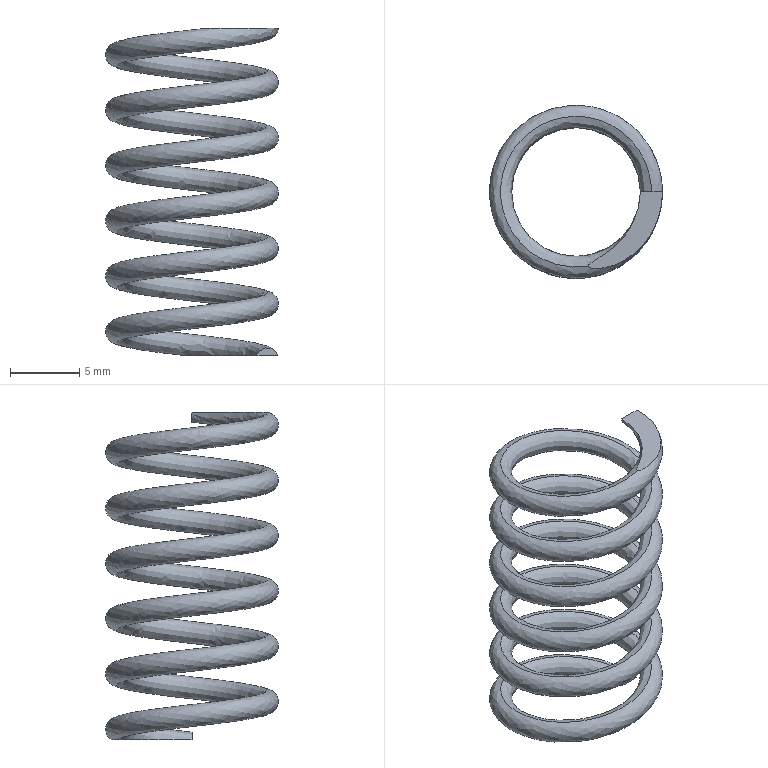Part | SolidWorks | features BaseBody 1 | 1 solid | 6 faces | box 12.495 x 12.5 x 23.645 mm | volume 403.779 mm3 | plane 4 | spline 2